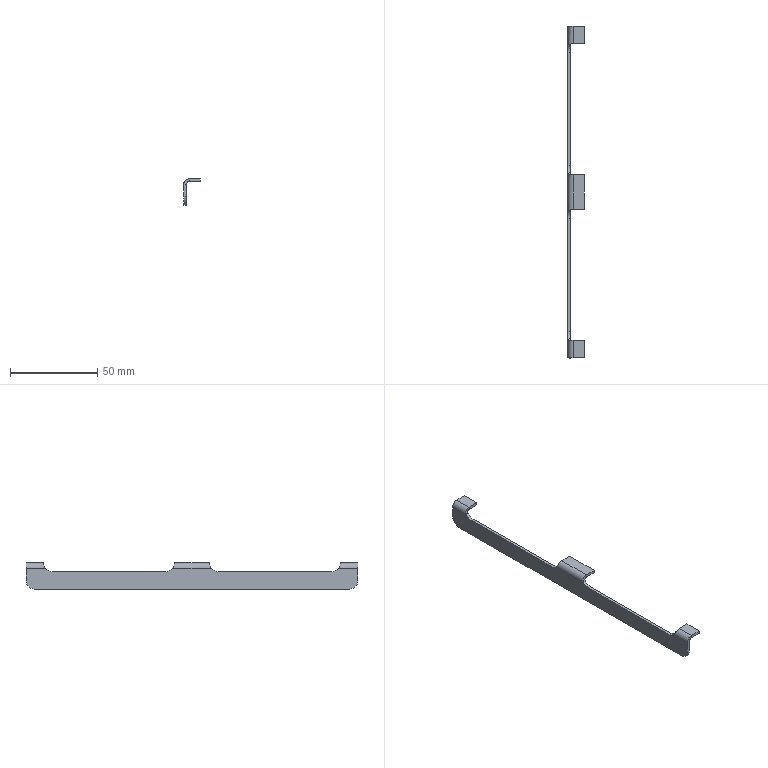Part | SolidWorks | features ICE 2, FlatPattern 1, SMBaseFlange 1, SheetMetal 1 | 1 solid | 40 faces | box 9.6 x 190 x 15 mm | volume 3822 mm3 | plane 24 | cylinder 12 | spline 4 | commonest cylinder face diameters 10 x6 3.2 x3 6.4 x3